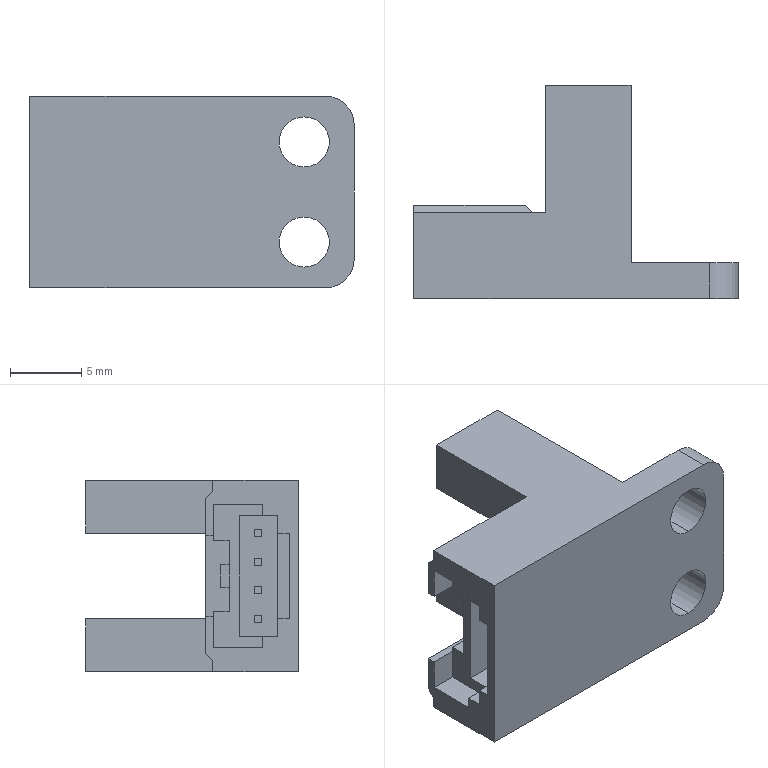Part | STEP file | Photoelectric sensor PM-Y65 | 1 solid | 107 faces | box 22.7 x 14.9 x 13.4 mm | volume 1660 mm3 | plane 101 | cylinder 6 | commonest cylinder face diameters 3.5 x4 4 x2